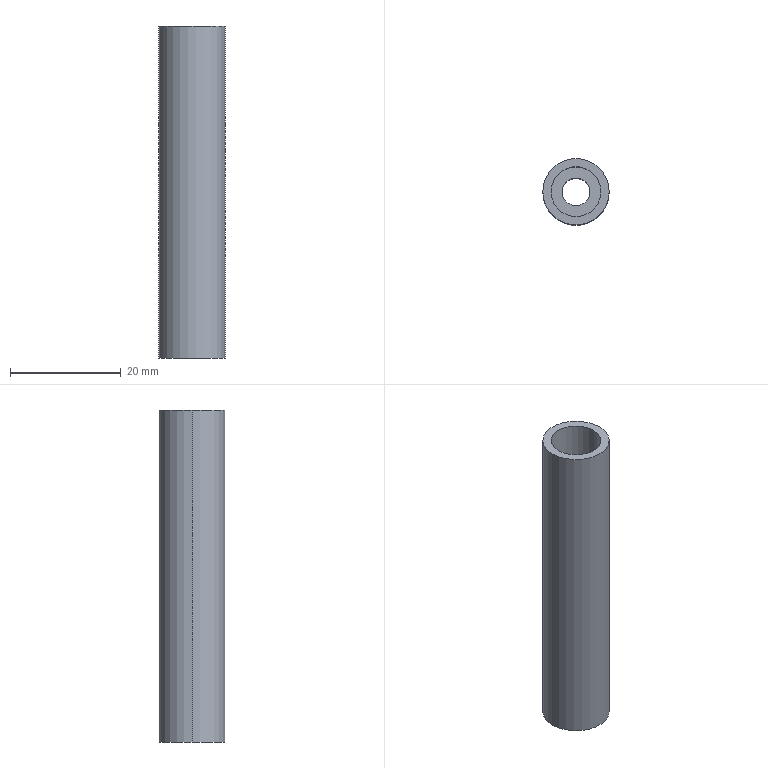Part | STEP file | Handle A | 1 solid | 9 faces | box 12 x 12 x 60 mm | volume 5168 mm3 | cylinder 6 | plane 3 | commonest cylinder face diameters 5 x2 9 x2 12 x2
STEP:
#1=CARTESIAN_POINT('',(0.,0.,0.));
#2=DIRECTION('',(0.,0.,1.));
#3=DIRECTION('',(1.,0.,0.));
#4=AXIS2_PLACEMENT_3D('',#1,#2,#3);
#5=CARTESIAN_POINT('',(4.5,0.,20.));
#6=VERTEX_POINT('',#5);
#7=CARTESIAN_POINT('',(4.5,0.,30.));
#8=VERTEX_POINT('',#7);
#9=CARTESIAN_POINT('',(4.5,0.,20.));
#10=DIRECTION('',(0.,0.,1.));
#11=VECTOR('',#10,1.);
#12=LINE('',#9,#11);
#13=CARTESIAN_POINT('',(0.,0.,20.));
#14=DIRECTION('',(0.,0.,1.));
#15=DIRECTION('',(1.,0.,0.));
#16=AXIS2_PLACEMENT_3D('',#13,#14,#15);
#17=CYLINDRICAL_SURFACE('',#16,4.5);
#18=CARTESIAN_POINT('',(6.283,0.));
#19=DIRECTION('',(0.,1.));
#20=VECTOR('',#19,1.);
#21=LINE('',#18,#20);
#22=(GEOMETRIC_REPRESENTATION_CONTEXT(2)PARAMETRIC_REPRESENTATION_CONTEXT()REPRESENTATION_CONTEXT('',''));
#23=DEFINITIONAL_REPRESENTATION('',(#21),#22);
#24=PCURVE('',#17,#23);
#25=CARTESIAN_POINT('',(0.,0.,20.));
#26=DIRECTION('',(0.,0.,1.));
#27=DIRECTION('',(1.,0.,0.));
#28=AXIS2_PLACEMENT_3D('',#25,#26,#27);
#29=CYLINDRICAL_SURFACE('',#28,4.5);
#30=CARTESIAN_POINT('',(0.,0.));
#31=DIRECTION('',(0.,1.));
#32=VECTOR('',#31,1.);
#33=LINE('',#30,#32);
#34=(GEOMETRIC_REPRESENTATION_CONTEXT(2)PARAMETRIC_REPRESENTATION_CONTEXT()REPRESENTATION_CONTEXT('',''));
#35=DEFINITIONAL_REPRESENTATION('',(#33),#34);
#36=PCURVE('',#29,#35);
#37=SURFACE_CURVE('',#12,(#24,#36),.PCURVE_S1.);
#38=EDGE_CURVE('',#6,#8,#37,.T.);
#39=ORIENTED_EDGE('',*,*,#38,.T.);
#40=CARTESIAN_POINT('',(-4.5,0.,30.));
#41=VERTEX_POINT('',#40);
#42=CARTESIAN_POINT('',(0.,0.,30.));
#43=DIRECTION('',(0.,0.,1.));
#44=DIRECTION('',(1.,0.,0.));
#45=AXIS2_PLACEMENT_3D('',#42,#43,#44);
#46=CIRCLE('',#45,4.5);
#47=CARTESIAN_POINT('',(0.,10.));
#48=DIRECTION('',(1.,0.));
#49=VECTOR('',#48,1.);
#50=LINE('',#47,#49);
#51=(GEOMETRIC_REPRESENTATION_CONTEXT(2)PARAMETRIC_REPRESENTATION_CONTEXT()REPRESENTATION_CONTEXT('',''));
#52=DEFINITIONAL_REPRESENTATION('',(#50),#51);
#53=PCURVE('',#17,#52);
#54=CARTESIAN_POINT('',(0.,0.,30.));
#55=DIRECTION('',(0.,0.,1.));
#56=DIRECTION('',(1.,0.,0.));
#57=AXIS2_PLACEMENT_3D('',#54,#55,#56);
#58=PLANE('',#57);
#59=CARTESIAN_POINT('',(0.,0.));
#60=DIRECTION('',(1.,0.));
#61=AXIS2_PLACEMENT_2D('',#59,#60);
#62=CIRCLE('',#61,4.5);
#63=(GEOMETRIC_REPRESENTATION_CONTEXT(2)PARAMETRIC_REPRESENTATION_CONTEXT()REPRESENTATION_CONTEXT('',''));
#64=DEFINITIONAL_REPRESENTATION('',(#62),#63);
#65=PCURVE('',#58,#64);
#66=SURFACE_CURVE('',#46,(#53,#65),.PCURVE_S1.);
#67=EDGE_CURVE('',#41,#8,#66,.T.);
#68=ORIENTED_EDGE('',*,*,#67,.F.);
#69=CARTESIAN_POINT('',(-4.5,0.,20.));
#70=VERTEX_POINT('',#69);
#71=CARTESIAN_POINT('',(-4.5,0.,20.));
#72=DIRECTION('',(0.,0.,1.));
#73=VECTOR('',#72,1.);
#74=LINE('',#71,#73);
#75=CARTESIAN_POINT('',(3.142,0.));
#76=DIRECTION('',(0.,1.));
#77=VECTOR('',#76,1.);
#78=LINE('',#75,#77);
#79=(GEOMETRIC_REPRESENTATION_CONTEXT(2)PARAMETRIC_REPRESENTATION_CONTEXT()REPRESENTATION_CONTEXT('',''));
#80=DEFINITIONAL_REPRESENTATION('',(#78),#79);
#81=PCURVE('',#17,#80);
#82=CARTESIAN_POINT('',(3.142,0.));
#83=DIRECTION('',(0.,1.));
#84=VECTOR('',#83,1.);
#85=LINE('',#82,#84);
#86=(GEOMETRIC_REPRESENTATION_CONTEXT(2)PARAMETRIC_REPRESENTATION_CONTEXT()REPRESENTATION_CONTEXT('',''));
#87=DEFINITIONAL_REPRESENTATION('',(#85),#86);
#88=PCURVE('',#29,#87);
#89=SURFACE_CURVE('',#74,(#81,#88),.PCURVE_S1.);
#90=EDGE_CURVE('',#70,#41,#89,.T.);
#91=ORIENTED_EDGE('',*,*,#90,.F.);
#92=CARTESIAN_POINT('',(0.,0.,20.));
#93=DIRECTION('',(0.,0.,1.));
#94=DIRECTION('',(1.,0.,0.));
#95=AXIS2_PLACEMENT_3D('',#92,#93,#94);
#96=CIRCLE('',#95,4.5);
#97=CARTESIAN_POINT('',(0.,0.));
#98=DIRECTION('',(1.,0.));
#99=VECTOR('',#98,1.);
#100=LINE('',#97,#99);
#101=(GEOMETRIC_REPRESENTATION_CONTEXT(2)PARAMETRIC_REPRESENTATION_CONTEXT()REPRESENTATION_CONTEXT('',''));
#102=DEFINITIONAL_REPRESENTATION('',(#100),#101);
#103=PCURVE('',#17,#102);
#104=CARTESIAN_POINT('',(0.,0.,20.));
#105=DIRECTION('',(0.,0.,1.));
#106=DIRECTION('',(1.,0.,0.));
#107=AXIS2_PLACEMENT_3D('',#104,#105,#106);
#108=PLANE('',#107);
#109=CARTESIAN_POINT('',(0.,0.));
#110=DIRECTION('',(1.,0.));
#111=AXIS2_PLACEMENT_2D('',#109,#110);
#112=CIRCLE('',#111,4.5);
#113=(GEOMETRIC_REPRESENTATION_CONTEXT(2)PARAMETRIC_REPRESENTATION_CONTEXT()REPRESENTATION_CONTEXT('',''));
#114=DEFINITIONAL_REPRESENTATION('',(#112),#113);
#115=PCURVE('',#108,#114);
#116=SURFACE_CURVE('',#96,(#103,#115),.PCURVE_S1.);
#117=EDGE_CURVE('',#70,#6,#116,.T.);
#118=ORIENTED_EDGE('',*,*,#117,.T.);
#119=EDGE_LOOP('',(#39,#68,#91,#118));
#120=FACE_BOUND('',#119,.F.);
#121=ADVANCED_FACE('',(#120),#17,.F.);
#122=CARTESIAN_POINT('',(6.,0.,30.));
#123=VERTEX_POINT('',#122);
#124=CARTESIAN_POINT('',(-6.,0.,30.));
#125=VERTEX_POINT('',#124);
#126=CARTESIAN_POINT('',(0.,0.,30.));
#127=DIRECTION('',(0.,0.,1.));
#128=DIRECTION('',(1.,0.,0.));
#129=AXIS2_PLACEMENT_3D('',#126,#127,#128);
#130=CIRCLE('',#129,6.);
#131=CARTESIAN_POINT('',(0.,0.,30.));
#132=DIRECTION('',(0.,0.,-1.));
#133=DIRECTION('',(-1.,0.,0.));
#134=AXIS2_PLACEMENT_3D('',#131,#132,#133);
#135=CYLINDRICAL_SURFACE('',#134,6.);
#136=CARTESIAN_POINT('',(3.142,0.));
#137=DIRECTION('',(-1.,0.));
#138=VECTOR('',#137,1.);
#139=LINE('',#136,#138);
#140=(GEOMETRIC_REPRESENTATION_CONTEXT(2)PARAMETRIC_REPRESENTATION_CONTEXT()REPRESENTATION_CONTEXT('',''));
#141=DEFINITIONAL_REPRESENTATION('',(#139),#140);
#142=PCURVE('',#135,#141);
#143=CARTESIAN_POINT('',(0.,0.));
#144=DIRECTION('',(1.,0.));
#145=AXIS2_PLACEMENT_2D('',#143,#144);
#146=CIRCLE('',#145,6.);
#147=(GEOMETRIC_REPRESENTATION_CONTEXT(2)PARAMETRIC_REPRESENTATION_CONTEXT()REPRESENTATION_CONTEXT('',''));
#148=DEFINITIONAL_REPRESENTATION('',(#146),#147);
#149=PCURVE('',#58,#148);
#150=SURFACE_CURVE('',#130,(#142,#149),.PCURVE_S1.);
#151=EDGE_CURVE('',#123,#125,#150,.T.);
#152=ORIENTED_EDGE('',*,*,#151,.F.);
#153=CARTESIAN_POINT('',(6.,0.,-30.));
#154=VERTEX_POINT('',#153);
#155=CARTESIAN_POINT('',(6.,0.,30.));
#156=DIRECTION('',(0.,0.,-1.));
#157=VECTOR('',#156,1.);
#158=LINE('',#155,#157);
#159=CARTESIAN_POINT('',(3.142,0.));
#160=DIRECTION('',(0.,1.));
#161=VECTOR('',#160,1.);
#162=LINE('',#159,#161);
#163=(GEOMETRIC_REPRESENTATION_CONTEXT(2)PARAMETRIC_REPRESENTATION_CONTEXT()REPRESENTATION_CONTEXT('',''));
#164=DEFINITIONAL_REPRESENTATION('',(#162),#163);
#165=PCURVE('',#135,#164);
#166=CARTESIAN_POINT('',(0.,0.,30.));
#167=DIRECTION('',(0.,0.,-1.));
#168=DIRECTION('',(-1.,0.,0.));
#169=AXIS2_PLACEMENT_3D('',#166,#167,#168);
#170=CYLINDRICAL_SURFACE('',#169,6.);
#171=CARTESIAN_POINT('',(3.142,0.));
#172=DIRECTION('',(0.,1.));
#173=VECTOR('',#172,1.);
#174=LINE('',#171,#173);
#175=(GEOMETRIC_REPRESENTATION_CONTEXT(2)PARAMETRIC_REPRESENTATION_CONTEXT()REPRESENTATION_CONTEXT('',''));
#176=DEFINITIONAL_REPRESENTATION('',(#174),#175);
#177=PCURVE('',#170,#176);
#178=SURFACE_CURVE('',#158,(#165,#177),.PCURVE_S1.);
#179=EDGE_CURVE('',#123,#154,#178,.T.);
#180=ORIENTED_EDGE('',*,*,#179,.T.);
#181=CARTESIAN_POINT('',(-6.,0.,-30.));
#182=VERTEX_POINT('',#181);
#183=CARTESIAN_POINT('',(0.,0.,-30.));
#184=DIRECTION('',(0.,0.,1.));
#185=DIRECTION('',(1.,0.,0.));
#186=AXIS2_PLACEMENT_3D('',#183,#184,#185);
#187=CIRCLE('',#186,6.);
#188=CARTESIAN_POINT('',(3.142,60.));
#189=DIRECTION('',(-1.,0.));
#190=VECTOR('',#189,1.);
#191=LINE('',#188,#190);
#192=(GEOMETRIC_REPRESENTATION_CONTEXT(2)PARAMETRIC_REPRESENTATION_CONTEXT()REPRESENTATION_CONTEXT('',''));
#193=DEFINITIONAL_REPRESENTATION('',(#191),#192);
#194=PCURVE('',#135,#193);
#195=CARTESIAN_POINT('',(0.,0.,-30.));
#196=DIRECTION('',(0.,0.,1.));
#197=DIRECTION('',(1.,0.,0.));
#198=AXIS2_PLACEMENT_3D('',#195,#196,#197);
#199=PLANE('',#198);
#200=CARTESIAN_POINT('',(0.,0.));
#201=DIRECTION('',(1.,0.));
#202=AXIS2_PLACEMENT_2D('',#200,#201);
#203=CIRCLE('',#202,6.);
#204=(GEOMETRIC_REPRESENTATION_CONTEXT(2)PARAMETRIC_REPRESENTATION_CONTEXT()REPRESENTATION_CONTEXT('',''));
#205=DEFINITIONAL_REPRESENTATION('',(#203),#204);
#206=PCURVE('',#199,#205);
#207=SURFACE_CURVE('',#187,(#194,#206),.PCURVE_S1.);
#208=EDGE_CURVE('',#154,#182,#207,.T.);
#209=ORIENTED_EDGE('',*,*,#208,.T.);
#210=CARTESIAN_POINT('',(-6.,0.,30.));
#211=DIRECTION('',(0.,0.,-1.));
#212=VECTOR('',#211,1.);
#213=LINE('',#210,#212);
#214=CARTESIAN_POINT('',(0.,0.));
#215=DIRECTION('',(0.,1.));
#216=VECTOR('',#215,1.);
#217=LINE('',#214,#216);
#218=(GEOMETRIC_REPRESENTATION_CONTEXT(2)PARAMETRIC_REPRESENTATION_CONTEXT()REPRESENTATION_CONTEXT('',''));
#219=DEFINITIONAL_REPRESENTATION('',(#217),#218);
#220=PCURVE('',#135,#219);
#221=CARTESIAN_POINT('',(6.283,0.));
#222=DIRECTION('',(0.,1.));
#223=VECTOR('',#222,1.);
#224=LINE('',#221,#223);
#225=(GEOMETRIC_REPRESENTATION_CONTEXT(2)PARAMETRIC_REPRESENTATION_CONTEXT()REPRESENTATION_CONTEXT('',''));
#226=DEFINITIONAL_REPRESENTATION('',(#224),#225);
#227=PCURVE('',#170,#226);
#228=SURFACE_CURVE('',#213,(#220,#227),.PCURVE_S1.);
#229=EDGE_CURVE('',#125,#182,#228,.T.);
#230=ORIENTED_EDGE('',*,*,#229,.F.);
#231=EDGE_LOOP('',(#152,#180,#209,#230));
#232=FACE_BOUND('',#231,.T.);
#233=ADVANCED_FACE('',(#232),#135,.T.);
#234=CARTESIAN_POINT('',(-2.5,0.,20.));
#235=VERTEX_POINT('',#234);
#236=CARTESIAN_POINT('',(-2.5,0.,-30.));
#237=VERTEX_POINT('',#236);
#238=CARTESIAN_POINT('',(-2.5,0.,30.));
#239=DIRECTION('',(0.,0.,-1.));
#240=VECTOR('',#239,1.);
#241=LINE('',#238,#240);
#242=CARTESIAN_POINT('',(0.,0.,30.));
#243=DIRECTION('',(0.,0.,-1.));
#244=DIRECTION('',(-1.,0.,0.));
#245=AXIS2_PLACEMENT_3D('',#242,#243,#244);
#246=CYLINDRICAL_SURFACE('',#245,2.5);
#247=CARTESIAN_POINT('',(6.283,0.));
#248=DIRECTION('',(0.,1.));
#249=VECTOR('',#248,1.);
#250=LINE('',#247,#249);
#251=(GEOMETRIC_REPRESENTATION_CONTEXT(2)PARAMETRIC_REPRESENTATION_CONTEXT()REPRESENTATION_CONTEXT('',''));
#252=DEFINITIONAL_REPRESENTATION('',(#250),#251);
#253=PCURVE('',#246,#252);
#254=CARTESIAN_POINT('',(0.,0.,30.));
#255=DIRECTION('',(0.,0.,-1.));
#256=DIRECTION('',(-1.,0.,0.));
#257=AXIS2_PLACEMENT_3D('',#254,#255,#256);
#258=CYLINDRICAL_SURFACE('',#257,2.5);
#259=CARTESIAN_POINT('',(0.,0.));
#260=DIRECTION('',(0.,1.));
#261=VECTOR('',#260,1.);
#262=LINE('',#259,#261);
#263=(GEOMETRIC_REPRESENTATION_CONTEXT(2)PARAMETRIC_REPRESENTATION_CONTEXT()REPRESENTATION_CONTEXT('',''));
#264=DEFINITIONAL_REPRESENTATION('',(#262),#263);
#265=PCURVE('',#258,#264);
#266=SURFACE_CURVE('',#241,(#253,#265),.PCURVE_S1.);
#267=EDGE_CURVE('',#235,#237,#266,.T.);
#268=ORIENTED_EDGE('',*,*,#267,.T.);
#269=CARTESIAN_POINT('',(2.5,0.,-30.));
#270=VERTEX_POINT('',#269);
#271=CARTESIAN_POINT('',(0.,0.,-30.));
#272=DIRECTION('',(0.,0.,1.));
#273=DIRECTION('',(1.,0.,0.));
#274=AXIS2_PLACEMENT_3D('',#271,#272,#273);
#275=CIRCLE('',#274,2.5);
#276=CARTESIAN_POINT('',(9.425,60.));
#277=DIRECTION('',(-1.,0.));
#278=VECTOR('',#277,1.);
#279=LINE('',#276,#278);
#280=(GEOMETRIC_REPRESENTATION_CONTEXT(2)PARAMETRIC_REPRESENTATION_CONTEXT()REPRESENTATION_CONTEXT('',''));
#281=DEFINITIONAL_REPRESENTATION('',(#279),#280);
#282=PCURVE('',#246,#281);
#283=CARTESIAN_POINT('',(0.,0.));
#284=DIRECTION('',(1.,0.));
#285=AXIS2_PLACEMENT_2D('',#283,#284);
#286=CIRCLE('',#285,2.5);
#287=(GEOMETRIC_REPRESENTATION_CONTEXT(2)PARAMETRIC_REPRESENTATION_CONTEXT()REPRESENTATION_CONTEXT('',''));
#288=DEFINITIONAL_REPRESENTATION('',(#286),#287);
#289=PCURVE('',#199,#288);
#290=SURFACE_CURVE('',#275,(#282,#289),.PCURVE_S1.);
#291=EDGE_CURVE('',#237,#270,#290,.T.);
#292=ORIENTED_EDGE('',*,*,#291,.T.);
#293=CARTESIAN_POINT('',(2.5,0.,20.));
#294=VERTEX_POINT('',#293);
#295=CARTESIAN_POINT('',(2.5,0.,30.));
#296=DIRECTION('',(0.,0.,-1.));
#297=VECTOR('',#296,1.);
#298=LINE('',#295,#297);
#299=CARTESIAN_POINT('',(3.142,0.));
#300=DIRECTION('',(0.,1.));
#301=VECTOR('',#300,1.);
#302=LINE('',#299,#301);
#303=(GEOMETRIC_REPRESENTATION_CONTEXT(2)PARAMETRIC_REPRESENTATION_CONTEXT()REPRESENTATION_CONTEXT('',''));
#304=DEFINITIONAL_REPRESENTATION('',(#302),#303);
#305=PCURVE('',#246,#304);
#306=CARTESIAN_POINT('',(3.142,0.));
#307=DIRECTION('',(0.,1.));
#308=VECTOR('',#307,1.);
#309=LINE('',#306,#308);
#310=(GEOMETRIC_REPRESENTATION_CONTEXT(2)PARAMETRIC_REPRESENTATION_CONTEXT()REPRESENTATION_CONTEXT('',''));
#311=DEFINITIONAL_REPRESENTATION('',(#309),#310);
#312=PCURVE('',#258,#311);
#313=SURFACE_CURVE('',#298,(#305,#312),.PCURVE_S1.);
#314=EDGE_CURVE('',#294,#270,#313,.T.);
#315=ORIENTED_EDGE('',*,*,#314,.F.);
#316=CARTESIAN_POINT('',(0.,0.,20.));
#317=DIRECTION('',(0.,0.,1.));
#318=DIRECTION('',(1.,0.,0.));
#319=AXIS2_PLACEMENT_3D('',#316,#317,#318);
#320=CIRCLE('',#319,2.5);
#321=CARTESIAN_POINT('',(9.425,10.));
#322=DIRECTION('',(-1.,0.));
#323=VECTOR('',#322,1.);
#324=LINE('',#321,#323);
#325=(GEOMETRIC_REPRESENTATION_CONTEXT(2)PARAMETRIC_REPRESENTATION_CONTEXT()REPRESENTATION_CONTEXT('',''));
#326=DEFINITIONAL_REPRESENTATION('',(#324),#325);
#327=PCURVE('',#246,#326);
#328=CARTESIAN_POINT('',(0.,0.));
#329=DIRECTION('',(1.,0.));
#330=AXIS2_PLACEMENT_2D('',#328,#329);
#331=CIRCLE('',#330,2.5);
#332=(GEOMETRIC_REPRESENTATION_CONTEXT(2)PARAMETRIC_REPRESENTATION_CONTEXT()REPRESENTATION_CONTEXT('',''));
#333=DEFINITIONAL_REPRESENTATION('',(#331),#332);
#334=PCURVE('',#108,#333);
#335=SURFACE_CURVE('',#320,(#327,#334),.PCURVE_S1.);
#336=EDGE_CURVE('',#235,#294,#335,.T.);
#337=ORIENTED_EDGE('',*,*,#336,.F.);
#338=EDGE_LOOP('',(#268,#292,#315,#337));
#339=FACE_BOUND('',#338,.F.);
#340=ADVANCED_FACE('',(#339),#246,.F.);
#341=CARTESIAN_POINT('',(0.,0.,-30.));
#342=DIRECTION('',(0.,0.,1.));
#343=DIRECTION('',(1.,0.,0.));
#344=AXIS2_PLACEMENT_3D('',#341,#342,#343);
#345=CIRCLE('',#344,2.5);
#346=CARTESIAN_POINT('',(3.142,60.));
#347=DIRECTION('',(-1.,0.));
#348=VECTOR('',#347,1.);
#349=LINE('',#346,#348);
#350=(GEOMETRIC_REPRESENTATION_CONTEXT(2)PARAMETRIC_REPRESENTATION_CONTEXT()REPRESENTATION_CONTEXT('',''));
#351=DEFINITIONAL_REPRESENTATION('',(#349),#350);
#352=PCURVE('',#258,#351);
#353=CARTESIAN_POINT('',(0.,0.));
#354=DIRECTION('',(1.,0.));
#355=AXIS2_PLACEMENT_2D('',#353,#354);
#356=CIRCLE('',#355,2.5);
#357=(GEOMETRIC_REPRESENTATION_CONTEXT(2)PARAMETRIC_REPRESENTATION_CONTEXT()REPRESENTATION_CONTEXT('',''));
#358=DEFINITIONAL_REPRESENTATION('',(#356),#357);
#359=PCURVE('',#199,#358);
#360=SURFACE_CURVE('',#345,(#352,#359),.PCURVE_S1.);
#361=EDGE_CURVE('',#270,#237,#360,.T.);
#362=ORIENTED_EDGE('',*,*,#361,.T.);
#363=ORIENTED_EDGE('',*,*,#267,.F.);
#364=CARTESIAN_POINT('',(0.,0.,20.));
#365=DIRECTION('',(0.,0.,1.));
#366=DIRECTION('',(1.,0.,0.));
#367=AXIS2_PLACEMENT_3D('',#364,#365,#366);
#368=CIRCLE('',#367,2.5);
#369=CARTESIAN_POINT('',(3.142,10.));
#370=DIRECTION('',(-1.,0.));
#371=VECTOR('',#370,1.);
#372=LINE('',#369,#371);
#373=(GEOMETRIC_REPRESENTATION_CONTEXT(2)PARAMETRIC_REPRESENTATION_CONTEXT()REPRESENTATION_CONTEXT('',''));
#374=DEFINITIONAL_REPRESENTATION('',(#372),#373);
#375=PCURVE('',#258,#374);
#376=CARTESIAN_POINT('',(0.,0.));
#377=DIRECTION('',(1.,0.));
#378=AXIS2_PLACEMENT_2D('',#376,#377);
#379=CIRCLE('',#378,2.5);
#380=(GEOMETRIC_REPRESENTATION_CONTEXT(2)PARAMETRIC_REPRESENTATION_CONTEXT()REPRESENTATION_CONTEXT('',''));
#381=DEFINITIONAL_REPRESENTATION('',(#379),#380);
#382=PCURVE('',#108,#381);
#383=SURFACE_CURVE('',#368,(#375,#382),.PCURVE_S1.);
#384=EDGE_CURVE('',#294,#235,#383,.T.);
#385=ORIENTED_EDGE('',*,*,#384,.F.);
#386=ORIENTED_EDGE('',*,*,#314,.T.);
#387=EDGE_LOOP('',(#362,#363,#385,#386));
#388=FACE_BOUND('',#387,.F.);
#389=ADVANCED_FACE('',(#388),#258,.F.);
#390=CARTESIAN_POINT('',(0.,0.,30.));
#391=DIRECTION('',(0.,0.,1.));
#392=DIRECTION('',(1.,0.,0.));
#393=AXIS2_PLACEMENT_3D('',#390,#391,#392);
#394=CIRCLE('',#393,4.5);
#395=CARTESIAN_POINT('',(0.,0.));
#396=DIRECTION('',(1.,0.));
#397=AXIS2_PLACEMENT_2D('',#395,#396);
#398=CIRCLE('',#397,4.5);
#399=(GEOMETRIC_REPRESENTATION_CONTEXT(2)PARAMETRIC_REPRESENTATION_CONTEXT()REPRESENTATION_CONTEXT('',''));
#400=DEFINITIONAL_REPRESENTATION('',(#398),#399);
#401=PCURVE('',#58,#400);
#402=CARTESIAN_POINT('',(0.,10.));
#403=DIRECTION('',(1.,0.));
#404=VECTOR('',#403,1.);
#405=LINE('',#402,#404);
#406=(GEOMETRIC_REPRESENTATION_CONTEXT(2)PARAMETRIC_REPRESENTATION_CONTEXT()REPRESENTATION_CONTEXT('',''));
#407=DEFINITIONAL_REPRESENTATION('',(#405),#406);
#408=PCURVE('',#29,#407);
#409=SURFACE_CURVE('',#394,(#401,#408),.PCURVE_S1.);
#410=EDGE_CURVE('',#8,#41,#409,.T.);
#411=ORIENTED_EDGE('',*,*,#410,.F.);
#412=ORIENTED_EDGE('',*,*,#67,.F.);
#413=EDGE_LOOP('',(#411,#412));
#414=FACE_BOUND('',#413,.T.);
#415=CARTESIAN_POINT('',(0.,0.,30.));
#416=DIRECTION('',(0.,0.,1.));
#417=DIRECTION('',(1.,0.,0.));
#418=AXIS2_PLACEMENT_3D('',#415,#416,#417);
#419=CIRCLE('',#418,6.);
#420=CARTESIAN_POINT('',(0.,0.));
#421=DIRECTION('',(1.,0.));
#422=AXIS2_PLACEMENT_2D('',#420,#421);
#423=CIRCLE('',#422,6.);
#424=(GEOMETRIC_REPRESENTATION_CONTEXT(2)PARAMETRIC_REPRESENTATION_CONTEXT()REPRESENTATION_CONTEXT('',''));
#425=DEFINITIONAL_REPRESENTATION('',(#423),#424);
#426=PCURVE('',#58,#425);
#427=CARTESIAN_POINT('',(9.425,0.));
#428=DIRECTION('',(-1.,0.));
#429=VECTOR('',#428,1.);
#430=LINE('',#427,#429);
#431=(GEOMETRIC_REPRESENTATION_CONTEXT(2)PARAMETRIC_REPRESENTATION_CONTEXT()REPRESENTATION_CONTEXT('',''));
#432=DEFINITIONAL_REPRESENTATION('',(#430),#431);
#433=PCURVE('',#170,#432);
#434=SURFACE_CURVE('',#419,(#426,#433),.PCURVE_S1.);
#435=EDGE_CURVE('',#125,#123,#434,.T.);
#436=ORIENTED_EDGE('',*,*,#435,.T.);
#437=ORIENTED_EDGE('',*,*,#151,.T.);
#438=EDGE_LOOP('',(#436,#437));
#439=FACE_BOUND('',#438,.T.);
#440=ADVANCED_FACE('',(#414,#439),#58,.T.);
#441=CARTESIAN_POINT('',(0.,0.,-30.));
#442=DIRECTION('',(0.,0.,1.));
#443=DIRECTION('',(1.,0.,0.));
#444=AXIS2_PLACEMENT_3D('',#441,#442,#443);
#445=CIRCLE('',#444,6.);
#446=CARTESIAN_POINT('',(0.,0.));
#447=DIRECTION('',(1.,0.));
#448=AXIS2_PLACEMENT_2D('',#446,#447);
#449=CIRCLE('',#448,6.);
#450=(GEOMETRIC_REPRESENTATION_CONTEXT(2)PARAMETRIC_REPRESENTATION_CONTEXT()REPRESENTATION_CONTEXT('',''));
#451=DEFINITIONAL_REPRESENTATION('',(#449),#450);
#452=PCURVE('',#199,#451);
#453=CARTESIAN_POINT('',(9.425,60.));
#454=DIRECTION('',(-1.,0.));
#455=VECTOR('',#454,1.);
#456=LINE('',#453,#455);
#457=(GEOMETRIC_REPRESENTATION_CONTEXT(2)PARAMETRIC_REPRESENTATION_CONTEXT()REPRESENTATION_CONTEXT('',''));
#458=DEFINITIONAL_REPRESENTATION('',(#456),#457);
#459=PCURVE('',#170,#458);
#460=SURFACE_CURVE('',#445,(#452,#459),.PCURVE_S1.);
#461=EDGE_CURVE('',#182,#154,#460,.T.);
#462=ORIENTED_EDGE('',*,*,#461,.F.);
#463=ORIENTED_EDGE('',*,*,#208,.F.);
#464=EDGE_LOOP('',(#462,#463));
#465=FACE_BOUND('',#464,.T.);
#466=ORIENTED_EDGE('',*,*,#291,.T.);
#467=ORIENTED_EDGE('',*,*,#361,.T.);
#468=EDGE_LOOP('',(#466,#467));
#469=FACE_BOUND('',#468,.T.);
#470=ADVANCED_FACE('',(#465,#469),#199,.F.);
#471=ORIENTED_EDGE('',*,*,#179,.F.);
#472=ORIENTED_EDGE('',*,*,#435,.F.);
#473=ORIENTED_EDGE('',*,*,#229,.T.);
#474=ORIENTED_EDGE('',*,*,#461,.T.);
#475=EDGE_LOOP('',(#471,#472,#473,#474));
#476=FACE_BOUND('',#475,.T.);
#477=ADVANCED_FACE('',(#476),#170,.T.);
#478=ORIENTED_EDGE('',*,*,#410,.F.);
#479=ORIENTED_EDGE('',*,*,#38,.F.);
#480=CARTESIAN_POINT('',(0.,0.,20.));
#481=DIRECTION('',(0.,0.,1.));
#482=DIRECTION('',(1.,0.,0.));
#483=AXIS2_PLACEMENT_3D('',#480,#481,#482);
#484=CIRCLE('',#483,4.5);
#485=CARTESIAN_POINT('',(0.,0.));
#486=DIRECTION('',(1.,0.));
#487=VECTOR('',#486,1.);
#488=LINE('',#485,#487);
#489=(GEOMETRIC_REPRESENTATION_CONTEXT(2)PARAMETRIC_REPRESENTATION_CONTEXT()REPRESENTATION_CONTEXT('',''));
#490=DEFINITIONAL_REPRESENTATION('',(#488),#489);
#491=PCURVE('',#29,#490);
#492=CARTESIAN_POINT('',(0.,0.));
#493=DIRECTION('',(1.,0.));
#494=AXIS2_PLACEMENT_2D('',#492,#493);
#495=CIRCLE('',#494,4.5);
#496=(GEOMETRIC_REPRESENTATION_CONTEXT(2)PARAMETRIC_REPRESENTATION_CONTEXT()REPRESENTATION_CONTEXT('',''));
#497=DEFINITIONAL_REPRESENTATION('',(#495),#496);
#498=PCURVE('',#108,#497);
#499=SURFACE_CURVE('',#484,(#491,#498),.PCURVE_S1.);
#500=EDGE_CURVE('',#6,#70,#499,.T.);
#501=ORIENTED_EDGE('',*,*,#500,.T.);
#502=ORIENTED_EDGE('',*,*,#90,.T.);
#503=EDGE_LOOP('',(#478,#479,#501,#502));
#504=FACE_BOUND('',#503,.F.);
#505=ADVANCED_FACE('',(#504),#29,.F.);
#506=ORIENTED_EDGE('',*,*,#336,.F.);
#507=ORIENTED_EDGE('',*,*,#384,.F.);
#508=EDGE_LOOP('',(#506,#507));
#509=FACE_BOUND('',#508,.T.);
#510=ORIENTED_EDGE('',*,*,#500,.T.);
#511=ORIENTED_EDGE('',*,*,#117,.T.);
#512=EDGE_LOOP('',(#510,#511));
#513=FACE_BOUND('',#512,.T.);
#514=ADVANCED_FACE('',(#509,#513),#108,.T.);
#515=CLOSED_SHELL('',(#121,#233,#340,#389,#440,#470,#477,#505,#514));
#516=MANIFOLD_SOLID_BREP('',#515);
#517=(LENGTH_UNIT()NAMED_UNIT(*)SI_UNIT(.MILLI.,.METRE.));
#518=UNCERTAINTY_MEASURE_WITH_UNIT(LENGTH_MEASURE(0.0000001),#517,'','');
#519=(NAMED_UNIT(*)PLANE_ANGLE_UNIT()SI_UNIT($,.RADIAN.));
#520=(NAMED_UNIT(*)SI_UNIT($,.STERADIAN.)SOLID_ANGLE_UNIT());
#521=(GEOMETRIC_REPRESENTATION_CONTEXT(3)GLOBAL_UNCERTAINTY_ASSIGNED_CONTEXT((#518))GLOBAL_UNIT_ASSIGNED_CONTEXT((#517,#519,#520))REPRESENTATION_CONTEXT('',''));
#522=ADVANCED_BREP_SHAPE_REPRESENTATION('',(#4,#516),#521);